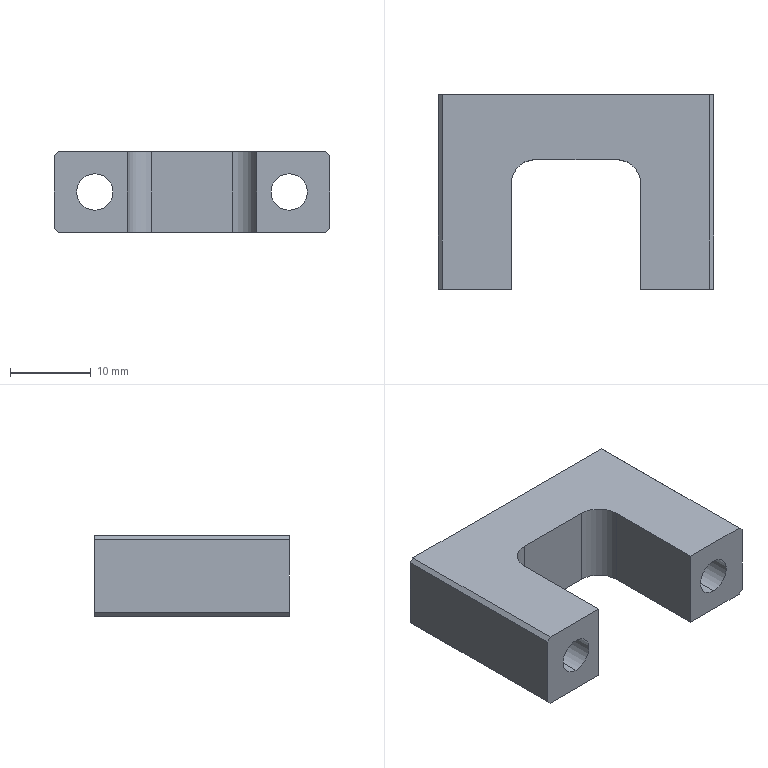Part | SolidWorks | features BaseBody 1 | 1 solid | 26 faces | box 34 x 24 x 10 mm | volume 4547 mm3 | plane 16 | cylinder 10 | commonest cylinder face diameters 4.5 x4 8 x4 6 x2
STEP:
#1=CARTESIAN_POINT('',(-12.,-4.6,-4.));
#2=VERTEX_POINT('',#1);
#3=CARTESIAN_POINT('',(-12.,-4.6,4.));
#4=VERTEX_POINT('',#3);
#5=CARTESIAN_POINT('',(-12.,-4.6,0.));
#6=DIRECTION('',(0.,1.,0.));
#7=DIRECTION('',(0.,0.,1.));
#8=AXIS2_PLACEMENT_3D('',#5,#6,#7);
#9=CIRCLE('',#8,4.);
#10=EDGE_CURVE('',#2,#4,#9,.T.);
#11=ORIENTED_EDGE('',*,*,#10,.F.);
#12=CARTESIAN_POINT('',(-12.,0.,-4.));
#13=VERTEX_POINT('',#12);
#14=CARTESIAN_POINT('',(-12.,0.,-4.));
#15=DIRECTION('',(0.,1.,0.));
#16=VECTOR('',#15,1000.);
#17=LINE('',#14,#16);
#18=EDGE_CURVE('',#2,#13,#17,.T.);
#19=ORIENTED_EDGE('',*,*,#18,.T.);
#20=CARTESIAN_POINT('',(-12.,0.,4.));
#21=VERTEX_POINT('',#20);
#22=CARTESIAN_POINT('',(-12.,0.,0.));
#23=DIRECTION('',(0.,1.,0.));
#24=DIRECTION('',(0.,0.,1.));
#25=AXIS2_PLACEMENT_3D('',#22,#23,#24);
#26=CIRCLE('',#25,4.);
#27=EDGE_CURVE('',#13,#21,#26,.T.);
#28=ORIENTED_EDGE('',*,*,#27,.T.);
#29=CARTESIAN_POINT('',(-12.,0.,4.));
#30=DIRECTION('',(0.,1.,0.));
#31=VECTOR('',#30,1000.);
#32=LINE('',#29,#31);
#33=EDGE_CURVE('',#4,#21,#32,.T.);
#34=ORIENTED_EDGE('',*,*,#33,.F.);
#35=EDGE_LOOP('',(#11,#19,#28,#34));
#36=FACE_OUTER_BOUND('',#35,.T.);
#37=CARTESIAN_POINT('',(-12.,0.,0.));
#38=DIRECTION('',(0.,1.,0.));
#39=DIRECTION('',(0.,0.,1.));
#40=AXIS2_PLACEMENT_3D('',#37,#38,#39);
#41=CYLINDRICAL_SURFACE('',#40,4.);
#42=ADVANCED_FACE('',(#36),#41,.F.);
#43=CARTESIAN_POINT('',(-12.,-24.,-2.25));
#44=VERTEX_POINT('',#43);
#45=CARTESIAN_POINT('',(-12.,-24.,2.25));
#46=VERTEX_POINT('',#45);
#47=CARTESIAN_POINT('',(-12.,-24.,0.));
#48=DIRECTION('',(0.,1.,0.));
#49=DIRECTION('',(-1.,0.,0.));
#50=AXIS2_PLACEMENT_3D('',#47,#48,#49);
#51=CIRCLE('',#50,2.25);
#52=EDGE_CURVE('',#44,#46,#51,.T.);
#53=ORIENTED_EDGE('',*,*,#52,.F.);
#54=CARTESIAN_POINT('',(-12.,-4.6,-2.25));
#55=VERTEX_POINT('',#54);
#56=CARTESIAN_POINT('',(-12.,0.,-2.25));
#57=DIRECTION('',(0.,1.,0.));
#58=VECTOR('',#57,1000.);
#59=LINE('',#56,#58);
#60=EDGE_CURVE('',#44,#55,#59,.T.);
#61=ORIENTED_EDGE('',*,*,#60,.T.);
#62=CARTESIAN_POINT('',(-12.,-4.6,2.25));
#63=VERTEX_POINT('',#62);
#64=CARTESIAN_POINT('',(-12.,-4.6,0.));
#65=DIRECTION('',(0.,1.,0.));
#66=DIRECTION('',(0.,0.,1.));
#67=AXIS2_PLACEMENT_3D('',#64,#65,#66);
#68=CIRCLE('',#67,2.25);
#69=EDGE_CURVE('',#55,#63,#68,.T.);
#70=ORIENTED_EDGE('',*,*,#69,.T.);
#71=CARTESIAN_POINT('',(-12.,0.,2.25));
#72=DIRECTION('',(0.,1.,0.));
#73=VECTOR('',#72,1000.);
#74=LINE('',#71,#73);
#75=EDGE_CURVE('',#46,#63,#74,.T.);
#76=ORIENTED_EDGE('',*,*,#75,.F.);
#77=EDGE_LOOP('',(#53,#61,#70,#76));
#78=FACE_OUTER_BOUND('',#77,.T.);
#79=CARTESIAN_POINT('',(-12.,0.,0.));
#80=DIRECTION('',(0.,1.,0.));
#81=DIRECTION('',(0.,0.,1.));
#82=AXIS2_PLACEMENT_3D('',#79,#80,#81);
#83=CYLINDRICAL_SURFACE('',#82,2.25);
#84=ADVANCED_FACE('',(#78),#83,.F.);
#85=CARTESIAN_POINT('',(12.,-4.6,-4.));
#86=VERTEX_POINT('',#85);
#87=CARTESIAN_POINT('',(12.,-4.6,4.));
#88=VERTEX_POINT('',#87);
#89=CARTESIAN_POINT('',(12.,-4.6,0.));
#90=DIRECTION('',(0.,1.,0.));
#91=DIRECTION('',(0.,0.,1.));
#92=AXIS2_PLACEMENT_3D('',#89,#90,#91);
#93=CIRCLE('',#92,4.);
#94=EDGE_CURVE('',#86,#88,#93,.T.);
#95=ORIENTED_EDGE('',*,*,#94,.F.);
#96=CARTESIAN_POINT('',(12.,0.,-4.));
#97=VERTEX_POINT('',#96);
#98=CARTESIAN_POINT('',(12.,0.,-4.));
#99=DIRECTION('',(0.,1.,0.));
#100=VECTOR('',#99,1000.);
#101=LINE('',#98,#100);
#102=EDGE_CURVE('',#86,#97,#101,.T.);
#103=ORIENTED_EDGE('',*,*,#102,.T.);
#104=CARTESIAN_POINT('',(12.,0.,4.));
#105=VERTEX_POINT('',#104);
#106=CARTESIAN_POINT('',(12.,0.,0.));
#107=DIRECTION('',(0.,1.,0.));
#108=DIRECTION('',(0.,0.,1.));
#109=AXIS2_PLACEMENT_3D('',#106,#107,#108);
#110=CIRCLE('',#109,4.);
#111=EDGE_CURVE('',#97,#105,#110,.T.);
#112=ORIENTED_EDGE('',*,*,#111,.T.);
#113=CARTESIAN_POINT('',(12.,0.,4.));
#114=DIRECTION('',(0.,1.,0.));
#115=VECTOR('',#114,1000.);
#116=LINE('',#113,#115);
#117=EDGE_CURVE('',#88,#105,#116,.T.);
#118=ORIENTED_EDGE('',*,*,#117,.F.);
#119=EDGE_LOOP('',(#95,#103,#112,#118));
#120=FACE_OUTER_BOUND('',#119,.T.);
#121=CARTESIAN_POINT('',(12.,0.,0.));
#122=DIRECTION('',(0.,1.,0.));
#123=DIRECTION('',(0.,0.,1.));
#124=AXIS2_PLACEMENT_3D('',#121,#122,#123);
#125=CYLINDRICAL_SURFACE('',#124,4.);
#126=ADVANCED_FACE('',(#120),#125,.F.);
#127=CARTESIAN_POINT('',(12.,-24.,-2.25));
#128=VERTEX_POINT('',#127);
#129=CARTESIAN_POINT('',(12.,-24.,2.25));
#130=VERTEX_POINT('',#129);
#131=CARTESIAN_POINT('',(12.,-24.,0.));
#132=DIRECTION('',(0.,1.,0.));
#133=DIRECTION('',(-1.,0.,0.));
#134=AXIS2_PLACEMENT_3D('',#131,#132,#133);
#135=CIRCLE('',#134,2.25);
#136=EDGE_CURVE('',#128,#130,#135,.T.);
#137=ORIENTED_EDGE('',*,*,#136,.F.);
#138=CARTESIAN_POINT('',(12.,-4.6,-2.25));
#139=VERTEX_POINT('',#138);
#140=CARTESIAN_POINT('',(12.,0.,-2.25));
#141=DIRECTION('',(0.,1.,0.));
#142=VECTOR('',#141,1000.);
#143=LINE('',#140,#142);
#144=EDGE_CURVE('',#128,#139,#143,.T.);
#145=ORIENTED_EDGE('',*,*,#144,.T.);
#146=CARTESIAN_POINT('',(12.,-4.6,2.25));
#147=VERTEX_POINT('',#146);
#148=CARTESIAN_POINT('',(12.,-4.6,0.));
#149=DIRECTION('',(0.,1.,0.));
#150=DIRECTION('',(0.,0.,1.));
#151=AXIS2_PLACEMENT_3D('',#148,#149,#150);
#152=CIRCLE('',#151,2.25);
#153=EDGE_CURVE('',#139,#147,#152,.T.);
#154=ORIENTED_EDGE('',*,*,#153,.T.);
#155=CARTESIAN_POINT('',(12.,0.,2.25));
#156=DIRECTION('',(0.,1.,0.));
#157=VECTOR('',#156,1000.);
#158=LINE('',#155,#157);
#159=EDGE_CURVE('',#130,#147,#158,.T.);
#160=ORIENTED_EDGE('',*,*,#159,.F.);
#161=EDGE_LOOP('',(#137,#145,#154,#160));
#162=FACE_OUTER_BOUND('',#161,.T.);
#163=CARTESIAN_POINT('',(12.,0.,0.));
#164=DIRECTION('',(0.,1.,0.));
#165=DIRECTION('',(0.,0.,1.));
#166=AXIS2_PLACEMENT_3D('',#163,#164,#165);
#167=CYLINDRICAL_SURFACE('',#166,2.25);
#168=ADVANCED_FACE('',(#162),#167,.F.);
#169=CARTESIAN_POINT('',(-8.,-11.,5.));
#170=VERTEX_POINT('',#169);
#171=CARTESIAN_POINT('',(-5.,-8.,5.));
#172=VERTEX_POINT('',#171);
#173=CARTESIAN_POINT('',(-5.,-11.,5.));
#174=DIRECTION('',(0.,0.,-1.));
#175=DIRECTION('',(-1.,0.,0.));
#176=AXIS2_PLACEMENT_3D('',#173,#174,#175);
#177=CIRCLE('',#176,3.);
#178=EDGE_CURVE('',#170,#172,#177,.T.);
#179=ORIENTED_EDGE('',*,*,#178,.F.);
#180=CARTESIAN_POINT('',(-8.,-11.,-5.));
#181=VERTEX_POINT('',#180);
#182=CARTESIAN_POINT('',(-8.,-11.,5.));
#183=DIRECTION('',(0.,0.,1.));
#184=VECTOR('',#183,1000.);
#185=LINE('',#182,#184);
#186=EDGE_CURVE('',#181,#170,#185,.T.);
#187=ORIENTED_EDGE('',*,*,#186,.F.);
#188=CARTESIAN_POINT('',(-5.,-8.,-5.));
#189=VERTEX_POINT('',#188);
#190=CARTESIAN_POINT('',(-5.,-11.,-5.));
#191=DIRECTION('',(0.,0.,1.));
#192=DIRECTION('',(-1.,0.,0.));
#193=AXIS2_PLACEMENT_3D('',#190,#191,#192);
#194=CIRCLE('',#193,3.);
#195=EDGE_CURVE('',#189,#181,#194,.T.);
#196=ORIENTED_EDGE('',*,*,#195,.F.);
#197=CARTESIAN_POINT('',(-5.,-8.,-5.));
#198=DIRECTION('',(0.,0.,-1.));
#199=VECTOR('',#198,1000.);
#200=LINE('',#197,#199);
#201=EDGE_CURVE('',#172,#189,#200,.T.);
#202=ORIENTED_EDGE('',*,*,#201,.F.);
#203=EDGE_LOOP('',(#179,#187,#196,#202));
#204=FACE_OUTER_BOUND('',#203,.T.);
#205=CARTESIAN_POINT('',(-5.,-11.,5.));
#206=DIRECTION('',(0.,0.,1.));
#207=DIRECTION('',(1.,0.,0.));
#208=AXIS2_PLACEMENT_3D('',#205,#206,#207);
#209=CYLINDRICAL_SURFACE('',#208,3.);
#210=ADVANCED_FACE('',(#204),#209,.F.);
#211=CARTESIAN_POINT('',(5.,-8.,5.));
#212=VERTEX_POINT('',#211);
#213=CARTESIAN_POINT('',(8.,-11.,5.));
#214=VERTEX_POINT('',#213);
#215=CARTESIAN_POINT('',(5.,-11.,5.));
#216=DIRECTION('',(0.,0.,-1.));
#217=DIRECTION('',(-1.,0.,0.));
#218=AXIS2_PLACEMENT_3D('',#215,#216,#217);
#219=CIRCLE('',#218,3.);
#220=EDGE_CURVE('',#212,#214,#219,.T.);
#221=ORIENTED_EDGE('',*,*,#220,.F.);
#222=CARTESIAN_POINT('',(5.,-8.,-5.));
#223=VERTEX_POINT('',#222);
#224=CARTESIAN_POINT('',(5.,-8.,5.));
#225=DIRECTION('',(0.,0.,1.));
#226=VECTOR('',#225,1000.);
#227=LINE('',#224,#226);
#228=EDGE_CURVE('',#223,#212,#227,.T.);
#229=ORIENTED_EDGE('',*,*,#228,.F.);
#230=CARTESIAN_POINT('',(8.,-11.,-5.));
#231=VERTEX_POINT('',#230);
#232=CARTESIAN_POINT('',(5.,-11.,-5.));
#233=DIRECTION('',(0.,0.,1.));
#234=DIRECTION('',(-1.,0.,0.));
#235=AXIS2_PLACEMENT_3D('',#232,#233,#234);
#236=CIRCLE('',#235,3.);
#237=EDGE_CURVE('',#231,#223,#236,.T.);
#238=ORIENTED_EDGE('',*,*,#237,.F.);
#239=CARTESIAN_POINT('',(8.,-11.,-5.));
#240=DIRECTION('',(0.,0.,-1.));
#241=VECTOR('',#240,1000.);
#242=LINE('',#239,#241);
#243=EDGE_CURVE('',#214,#231,#242,.T.);
#244=ORIENTED_EDGE('',*,*,#243,.F.);
#245=EDGE_LOOP('',(#221,#229,#238,#244));
#246=FACE_OUTER_BOUND('',#245,.T.);
#247=CARTESIAN_POINT('',(5.,-11.,5.));
#248=DIRECTION('',(0.,0.,1.));
#249=DIRECTION('',(1.,0.,0.));
#250=AXIS2_PLACEMENT_3D('',#247,#248,#249);
#251=CYLINDRICAL_SURFACE('',#250,3.);
#252=ADVANCED_FACE('',(#246),#251,.F.);
#253=CARTESIAN_POINT('',(-17.,0.,4.5));
#254=VERTEX_POINT('',#253);
#255=CARTESIAN_POINT('',(-16.5,0.,5.));
#256=VERTEX_POINT('',#255);
#257=CARTESIAN_POINT('',(-16.5,0.,5.));
#258=DIRECTION('',(0.7071,0.,0.7071));
#259=VECTOR('',#258,1000.);
#260=LINE('',#257,#259);
#261=EDGE_CURVE('',#254,#256,#260,.T.);
#262=ORIENTED_EDGE('',*,*,#261,.F.);
#263=CARTESIAN_POINT('',(-17.,-24.,4.5));
#264=VERTEX_POINT('',#263);
#265=CARTESIAN_POINT('',(-17.,-24.,4.5));
#266=DIRECTION('',(0.,1.,0.));
#267=VECTOR('',#266,1000.);
#268=LINE('',#265,#267);
#269=EDGE_CURVE('',#264,#254,#268,.T.);
#270=ORIENTED_EDGE('',*,*,#269,.F.);
#271=CARTESIAN_POINT('',(-16.5,-24.,5.));
#272=VERTEX_POINT('',#271);
#273=CARTESIAN_POINT('',(-16.5,-24.,5.));
#274=DIRECTION('',(-0.7071,0.,-0.7071));
#275=VECTOR('',#274,1000.);
#276=LINE('',#273,#275);
#277=EDGE_CURVE('',#272,#264,#276,.T.);
#278=ORIENTED_EDGE('',*,*,#277,.F.);
#279=CARTESIAN_POINT('',(-16.5,0.,5.));
#280=DIRECTION('',(0.,-1.,0.));
#281=VECTOR('',#280,1000.);
#282=LINE('',#279,#281);
#283=EDGE_CURVE('',#256,#272,#282,.T.);
#284=ORIENTED_EDGE('',*,*,#283,.F.);
#285=EDGE_LOOP('',(#262,#270,#278,#284));
#286=FACE_OUTER_BOUND('',#285,.T.);
#287=CARTESIAN_POINT('',(-16.5,0.,5.));
#288=DIRECTION('',(0.7071,0.,-0.7071));
#289=DIRECTION('',(0.,-1.,0.));
#290=AXIS2_PLACEMENT_3D('',#287,#288,#289);
#291=PLANE('',#290);
#292=ADVANCED_FACE('',(#286),#291,.F.);
#293=CARTESIAN_POINT('',(-16.5,0.,-5.));
#294=VERTEX_POINT('',#293);
#295=CARTESIAN_POINT('',(-17.,0.,-4.5));
#296=VERTEX_POINT('',#295);
#297=CARTESIAN_POINT('',(-17.,0.,-4.5));
#298=DIRECTION('',(-0.7071,0.,0.7071));
#299=VECTOR('',#298,1000.);
#300=LINE('',#297,#299);
#301=EDGE_CURVE('',#294,#296,#300,.T.);
#302=ORIENTED_EDGE('',*,*,#301,.F.);
#303=CARTESIAN_POINT('',(-16.5,-24.,-5.));
#304=VERTEX_POINT('',#303);
#305=CARTESIAN_POINT('',(-16.5,0.,-5.));
#306=DIRECTION('',(0.,1.,0.));
#307=VECTOR('',#306,1000.);
#308=LINE('',#305,#307);
#309=EDGE_CURVE('',#304,#294,#308,.T.);
#310=ORIENTED_EDGE('',*,*,#309,.F.);
#311=CARTESIAN_POINT('',(-17.,-24.,-4.5));
#312=VERTEX_POINT('',#311);
#313=CARTESIAN_POINT('',(-17.,-24.,-4.5));
#314=DIRECTION('',(0.7071,0.,-0.7071));
#315=VECTOR('',#314,1000.);
#316=LINE('',#313,#315);
#317=EDGE_CURVE('',#312,#304,#316,.T.);
#318=ORIENTED_EDGE('',*,*,#317,.F.);
#319=CARTESIAN_POINT('',(-17.,-24.,-4.5));
#320=DIRECTION('',(0.,-1.,0.));
#321=VECTOR('',#320,1000.);
#322=LINE('',#319,#321);
#323=EDGE_CURVE('',#296,#312,#322,.T.);
#324=ORIENTED_EDGE('',*,*,#323,.F.);
#325=EDGE_LOOP('',(#302,#310,#318,#324));
#326=FACE_OUTER_BOUND('',#325,.T.);
#327=CARTESIAN_POINT('',(-17.,-24.,-4.5));
#328=DIRECTION('',(-0.7071,0.,-0.7071));
#329=DIRECTION('',(-0.7071,0.,0.7071));
#330=AXIS2_PLACEMENT_3D('',#327,#328,#329);
#331=PLANE('',#330);
#332=ADVANCED_FACE('',(#326),#331,.T.);
#333=CARTESIAN_POINT('',(17.,-24.,4.5));
#334=VERTEX_POINT('',#333);
#335=CARTESIAN_POINT('',(16.5,-24.,5.));
#336=VERTEX_POINT('',#335);
#337=CARTESIAN_POINT('',(16.5,-24.,5.));
#338=DIRECTION('',(-0.7071,0.,0.7071));
#339=VECTOR('',#338,1000.);
#340=LINE('',#337,#339);
#341=EDGE_CURVE('',#334,#336,#340,.T.);
#342=ORIENTED_EDGE('',*,*,#341,.F.);
#343=CARTESIAN_POINT('',(17.,0.,4.5));
#344=VERTEX_POINT('',#343);
#345=CARTESIAN_POINT('',(17.,0.,4.5));
#346=DIRECTION('',(0.,-1.,0.));
#347=VECTOR('',#346,1000.);
#348=LINE('',#345,#347);
#349=EDGE_CURVE('',#344,#334,#348,.T.);
#350=ORIENTED_EDGE('',*,*,#349,.F.);
#351=CARTESIAN_POINT('',(16.5,0.,5.));
#352=VERTEX_POINT('',#351);
#353=CARTESIAN_POINT('',(16.5,0.,5.));
#354=DIRECTION('',(0.7071,0.,-0.7071));
#355=VECTOR('',#354,1000.);
#356=LINE('',#353,#355);
#357=EDGE_CURVE('',#352,#344,#356,.T.);
#358=ORIENTED_EDGE('',*,*,#357,.F.);
#359=CARTESIAN_POINT('',(16.5,0.,5.));
#360=DIRECTION('',(0.,1.,0.));
#361=VECTOR('',#360,1000.);
#362=LINE('',#359,#361);
#363=EDGE_CURVE('',#336,#352,#362,.T.);
#364=ORIENTED_EDGE('',*,*,#363,.F.);
#365=EDGE_LOOP('',(#342,#350,#358,#364));
#366=FACE_OUTER_BOUND('',#365,.T.);
#367=CARTESIAN_POINT('',(16.5,0.,5.));
#368=DIRECTION('',(-0.7071,0.,-0.7071));
#369=DIRECTION('',(-0.7071,0.,0.7071));
#370=AXIS2_PLACEMENT_3D('',#367,#368,#369);
#371=PLANE('',#370);
#372=ADVANCED_FACE('',(#366),#371,.F.);
#373=CARTESIAN_POINT('',(16.5,-24.,-5.));
#374=VERTEX_POINT('',#373);
#375=CARTESIAN_POINT('',(17.,-24.,-4.5));
#376=VERTEX_POINT('',#375);
#377=CARTESIAN_POINT('',(17.,-24.,-4.5));
#378=DIRECTION('',(0.7071,0.,0.7071));
#379=VECTOR('',#378,1000.);
#380=LINE('',#377,#379);
#381=EDGE_CURVE('',#374,#376,#380,.T.);
#382=ORIENTED_EDGE('',*,*,#381,.F.);
#383=CARTESIAN_POINT('',(16.5,0.,-5.));
#384=VERTEX_POINT('',#383);
#385=CARTESIAN_POINT('',(16.5,-24.,-5.));
#386=DIRECTION('',(0.,-1.,0.));
#387=VECTOR('',#386,1000.);
#388=LINE('',#385,#387);
#389=EDGE_CURVE('',#384,#374,#388,.T.);
#390=ORIENTED_EDGE('',*,*,#389,.F.);
#391=CARTESIAN_POINT('',(17.,0.,-4.5));
#392=VERTEX_POINT('',#391);
#393=CARTESIAN_POINT('',(17.,0.,-4.5));
#394=DIRECTION('',(-0.7071,0.,-0.7071));
#395=VECTOR('',#394,1000.);
#396=LINE('',#393,#395);
#397=EDGE_CURVE('',#392,#384,#396,.T.);
#398=ORIENTED_EDGE('',*,*,#397,.F.);
#399=CARTESIAN_POINT('',(17.,0.,-4.5));
#400=DIRECTION('',(0.,1.,0.));
#401=VECTOR('',#400,1000.);
#402=LINE('',#399,#401);
#403=EDGE_CURVE('',#376,#392,#402,.T.);
#404=ORIENTED_EDGE('',*,*,#403,.F.);
#405=EDGE_LOOP('',(#382,#390,#398,#404));
#406=FACE_OUTER_BOUND('',#405,.T.);
#407=CARTESIAN_POINT('',(17.,0.,-4.5));
#408=DIRECTION('',(0.7071,0.,-0.7071));
#409=DIRECTION('',(0.,-1.,0.));
#410=AXIS2_PLACEMENT_3D('',#407,#408,#409);
#411=PLANE('',#410);
#412=ADVANCED_FACE('',(#406),#411,.T.);
#413=CARTESIAN_POINT('',(-12.,-4.6,0.));
#414=DIRECTION('',(0.,1.,0.));
#415=DIRECTION('',(0.,0.,1.));
#416=AXIS2_PLACEMENT_3D('',#413,#414,#415);
#417=CIRCLE('',#416,2.25);
#418=EDGE_CURVE('',#63,#55,#417,.T.);
#419=ORIENTED_EDGE('',*,*,#418,.F.);
#420=ORIENTED_EDGE('',*,*,#69,.F.);
#421=EDGE_LOOP('',(#419,#420));
#422=FACE_BOUND('',#421,.T.);
#423=CARTESIAN_POINT('',(-12.,-4.6,0.));
#424=DIRECTION('',(0.,1.,0.));
#425=DIRECTION('',(0.,0.,1.));
#426=AXIS2_PLACEMENT_3D('',#423,#424,#425);
#427=CIRCLE('',#426,4.);
#428=EDGE_CURVE('',#4,#2,#427,.T.);
#429=ORIENTED_EDGE('',*,*,#428,.T.);
#430=ORIENTED_EDGE('',*,*,#10,.T.);
#431=EDGE_LOOP('',(#429,#430));
#432=FACE_OUTER_BOUND('',#431,.T.);
#433=CARTESIAN_POINT('',(-9.75,-4.6,0.));
#434=DIRECTION('',(0.,-1.,0.));
#435=DIRECTION('',(0.,0.,-1.));
#436=AXIS2_PLACEMENT_3D('',#433,#434,#435);
#437=PLANE('',#436);
#438=ADVANCED_FACE('',(#422,#432),#437,.F.);
#439=CARTESIAN_POINT('',(12.,-4.6,0.));
#440=DIRECTION('',(0.,1.,0.));
#441=DIRECTION('',(0.,0.,1.));
#442=AXIS2_PLACEMENT_3D('',#439,#440,#441);
#443=CIRCLE('',#442,2.25);
#444=EDGE_CURVE('',#147,#139,#443,.T.);
#445=ORIENTED_EDGE('',*,*,#444,.F.);
#446=ORIENTED_EDGE('',*,*,#153,.F.);
#447=EDGE_LOOP('',(#445,#446));
#448=FACE_BOUND('',#447,.T.);
#449=CARTESIAN_POINT('',(12.,-4.6,0.));
#450=DIRECTION('',(0.,1.,0.));
#451=DIRECTION('',(0.,0.,1.));
#452=AXIS2_PLACEMENT_3D('',#449,#450,#451);
#453=CIRCLE('',#452,4.);
#454=EDGE_CURVE('',#88,#86,#453,.T.);
#455=ORIENTED_EDGE('',*,*,#454,.T.);
#456=ORIENTED_EDGE('',*,*,#94,.T.);
#457=EDGE_LOOP('',(#455,#456));
#458=FACE_OUTER_BOUND('',#457,.T.);
#459=CARTESIAN_POINT('',(14.25,-4.6,0.));
#460=DIRECTION('',(0.,-1.,0.));
#461=DIRECTION('',(0.,0.,-1.));
#462=AXIS2_PLACEMENT_3D('',#459,#460,#461);
#463=PLANE('',#462);
#464=ADVANCED_FACE('',(#448,#458),#463,.F.);
#465=CARTESIAN_POINT('',(-17.,0.,-5.));
#466=DIRECTION('',(-1.,0.,0.));
#467=VECTOR('',#466,1000.);
#468=LINE('',#465,#467);
#469=EDGE_CURVE('',#384,#294,#468,.T.);
#470=ORIENTED_EDGE('',*,*,#469,.F.);
#471=ORIENTED_EDGE('',*,*,#389,.T.);
#472=CARTESIAN_POINT('',(8.,-24.,-5.));
#473=VERTEX_POINT('',#472);
#474=CARTESIAN_POINT('',(17.,-24.,-5.));
#475=DIRECTION('',(1.,0.,0.));
#476=VECTOR('',#475,1000.);
#477=LINE('',#474,#476);
#478=EDGE_CURVE('',#473,#374,#477,.T.);
#479=ORIENTED_EDGE('',*,*,#478,.F.);
#480=CARTESIAN_POINT('',(8.,-24.,-5.));
#481=DIRECTION('',(0.,-1.,0.));
#482=VECTOR('',#481,1000.);
#483=LINE('',#480,#482);
#484=EDGE_CURVE('',#231,#473,#483,.T.);
#485=ORIENTED_EDGE('',*,*,#484,.F.);
#486=ORIENTED_EDGE('',*,*,#237,.T.);
#487=CARTESIAN_POINT('',(8.,-8.,-5.));
#488=DIRECTION('',(1.,0.,0.));
#489=VECTOR('',#488,1000.);
#490=LINE('',#487,#489);
#491=EDGE_CURVE('',#189,#223,#490,.T.);
#492=ORIENTED_EDGE('',*,*,#491,.F.);
#493=ORIENTED_EDGE('',*,*,#195,.T.);
#494=CARTESIAN_POINT('',(-8.,-24.,-5.));
#495=VERTEX_POINT('',#494);
#496=CARTESIAN_POINT('',(-8.,-8.,-5.));
#497=DIRECTION('',(0.,1.,0.));
#498=VECTOR('',#497,1000.);
#499=LINE('',#496,#498);
#500=EDGE_CURVE('',#495,#181,#499,.T.);
#501=ORIENTED_EDGE('',*,*,#500,.F.);
#502=CARTESIAN_POINT('',(-8.,-24.,-5.));
#503=DIRECTION('',(1.,0.,0.));
#504=VECTOR('',#503,1000.);
#505=LINE('',#502,#504);
#506=EDGE_CURVE('',#304,#495,#505,.T.);
#507=ORIENTED_EDGE('',*,*,#506,.F.);
#508=ORIENTED_EDGE('',*,*,#309,.T.);
#509=EDGE_LOOP('',(#470,#471,#479,#485,#486,#492,#493,#501,#507,#508));
#510=FACE_OUTER_BOUND('',#509,.T.);
#511=CARTESIAN_POINT('',(0.,0.,-5.));
#512=DIRECTION('',(0.,0.,-1.));
#513=DIRECTION('',(0.,-1.,0.));
#514=AXIS2_PLACEMENT_3D('',#511,#512,#513);
#515=PLANE('',#514);
#516=ADVANCED_FACE('',(#510),#515,.T.);
#517=CARTESIAN_POINT('',(8.,-24.,5.));
#518=VERTEX_POINT('',#517);
#519=CARTESIAN_POINT('',(17.,-24.,5.));
#520=DIRECTION('',(1.,0.,0.));
#521=VECTOR('',#520,1000.);
#522=LINE('',#519,#521);
#523=EDGE_CURVE('',#518,#336,#522,.T.);
#524=ORIENTED_EDGE('',*,*,#523,.T.);
#525=ORIENTED_EDGE('',*,*,#363,.T.);
#526=CARTESIAN_POINT('',(-17.,0.,5.));
#527=DIRECTION('',(-1.,0.,0.));
#528=VECTOR('',#527,1000.);
#529=LINE('',#526,#528);
#530=EDGE_CURVE('',#352,#256,#529,.T.);
#531=ORIENTED_EDGE('',*,*,#530,.T.);
#532=ORIENTED_EDGE('',*,*,#283,.T.);
#533=CARTESIAN_POINT('',(-8.,-24.,5.));
#534=VERTEX_POINT('',#533);
#535=CARTESIAN_POINT('',(-8.,-24.,5.));
#536=DIRECTION('',(1.,0.,0.));
#537=VECTOR('',#536,1000.);
#538=LINE('',#535,#537);
#539=EDGE_CURVE('',#272,#534,#538,.T.);
#540=ORIENTED_EDGE('',*,*,#539,.T.);
#541=CARTESIAN_POINT('',(-8.,-8.,5.));
#542=DIRECTION('',(0.,1.,0.));
#543=VECTOR('',#542,1000.);
#544=LINE('',#541,#543);
#545=EDGE_CURVE('',#534,#170,#544,.T.);
#546=ORIENTED_EDGE('',*,*,#545,.T.);
#547=ORIENTED_EDGE('',*,*,#178,.T.);
#548=CARTESIAN_POINT('',(8.,-8.,5.));
#549=DIRECTION('',(1.,0.,0.));
#550=VECTOR('',#549,1000.);
#551=LINE('',#548,#550);
#552=EDGE_CURVE('',#172,#212,#551,.T.);
#553=ORIENTED_EDGE('',*,*,#552,.T.);
#554=ORIENTED_EDGE('',*,*,#220,.T.);
#555=CARTESIAN_POINT('',(8.,-24.,5.));
#556=DIRECTION('',(0.,-1.,0.));
#557=VECTOR('',#556,1000.);
#558=LINE('',#555,#557);
#559=EDGE_CURVE('',#214,#518,#558,.T.);
#560=ORIENTED_EDGE('',*,*,#559,.T.);
#561=EDGE_LOOP('',(#524,#525,#531,#532,#540,#546,#547,#553,#554,#560));
#562=FACE_OUTER_BOUND('',#561,.T.);
#563=CARTESIAN_POINT('',(0.,0.,5.));
#564=DIRECTION('',(0.,0.,-1.));
#565=DIRECTION('',(0.,-1.,0.));
#566=AXIS2_PLACEMENT_3D('',#563,#564,#565);
#567=PLANE('',#566);
#568=ADVANCED_FACE('',(#562),#567,.F.);
#569=CARTESIAN_POINT('',(-17.,0.,5.));
#570=DIRECTION('',(0.,0.,-1.));
#571=VECTOR('',#570,1000.);
#572=LINE('',#569,#571);
#573=EDGE_CURVE('',#254,#296,#572,.T.);
#574=ORIENTED_EDGE('',*,*,#573,.T.);
#575=ORIENTED_EDGE('',*,*,#323,.T.);
#576=CARTESIAN_POINT('',(-17.,-24.,5.));
#577=DIRECTION('',(0.,0.,-1.));
#578=VECTOR('',#577,1000.);
#579=LINE('',#576,#578);
#580=EDGE_CURVE('',#264,#312,#579,.T.);
#581=ORIENTED_EDGE('',*,*,#580,.F.);
#582=ORIENTED_EDGE('',*,*,#269,.T.);
#583=EDGE_LOOP('',(#574,#575,#581,#582));
#584=FACE_OUTER_BOUND('',#583,.T.);
#585=CARTESIAN_POINT('',(-17.,-24.,5.));
#586=DIRECTION('',(1.,0.,0.));
#587=DIRECTION('',(0.,1.,0.));
#588=AXIS2_PLACEMENT_3D('',#585,#586,#587);
#589=PLANE('',#588);
#590=ADVANCED_FACE('',(#584),#589,.F.);
#591=CARTESIAN_POINT('',(12.,0.,0.));
#592=DIRECTION('',(0.,1.,0.));
#593=DIRECTION('',(0.,0.,1.));
#594=AXIS2_PLACEMENT_3D('',#591,#592,#593);
#595=CIRCLE('',#594,4.);
#596=EDGE_CURVE('',#105,#97,#595,.T.);
#597=ORIENTED_EDGE('',*,*,#596,.F.);
#598=ORIENTED_EDGE('',*,*,#111,.F.);
#599=EDGE_LOOP('',(#597,#598));
#600=FACE_BOUND('',#599,.T.);
#601=CARTESIAN_POINT('',(-12.,0.,0.));
#602=DIRECTION('',(0.,1.,0.));
#603=DIRECTION('',(0.,0.,1.));
#604=AXIS2_PLACEMENT_3D('',#601,#602,#603);
#605=CIRCLE('',#604,4.);
#606=EDGE_CURVE('',#21,#13,#605,.T.);
#607=ORIENTED_EDGE('',*,*,#606,.F.);
#608=ORIENTED_EDGE('',*,*,#27,.F.);
#609=EDGE_LOOP('',(#607,#608));
#610=FACE_BOUND('',#609,.T.);
#611=CARTESIAN_POINT('',(17.,0.,5.));
#612=DIRECTION('',(0.,0.,-1.));
#613=VECTOR('',#612,1000.);
#614=LINE('',#611,#613);
#615=EDGE_CURVE('',#344,#392,#614,.T.);
#616=ORIENTED_EDGE('',*,*,#615,.T.);
#617=ORIENTED_EDGE('',*,*,#397,.T.);
#618=ORIENTED_EDGE('',*,*,#469,.T.);
#619=ORIENTED_EDGE('',*,*,#301,.T.);
#620=ORIENTED_EDGE('',*,*,#573,.F.);
#621=ORIENTED_EDGE('',*,*,#261,.T.);
#622=ORIENTED_EDGE('',*,*,#530,.F.);
#623=ORIENTED_EDGE('',*,*,#357,.T.);
#624=EDGE_LOOP('',(#616,#617,#618,#619,#620,#621,#622,#623));
#625=FACE_OUTER_BOUND('',#624,.T.);
#626=CARTESIAN_POINT('',(-17.,0.,5.));
#627=DIRECTION('',(0.,-1.,0.));
#628=DIRECTION('',(0.,0.,-1.));
#629=AXIS2_PLACEMENT_3D('',#626,#627,#628);
#630=PLANE('',#629);
#631=ADVANCED_FACE('',(#600,#610,#625),#630,.F.);
#632=CARTESIAN_POINT('',(17.,-24.,5.));
#633=DIRECTION('',(0.,0.,-1.));
#634=VECTOR('',#633,1000.);
#635=LINE('',#632,#634);
#636=EDGE_CURVE('',#334,#376,#635,.T.);
#637=ORIENTED_EDGE('',*,*,#636,.T.);
#638=ORIENTED_EDGE('',*,*,#403,.T.);
#639=ORIENTED_EDGE('',*,*,#615,.F.);
#640=ORIENTED_EDGE('',*,*,#349,.T.);
#641=EDGE_LOOP('',(#637,#638,#639,#640));
#642=FACE_OUTER_BOUND('',#641,.T.);
#643=CARTESIAN_POINT('',(17.,0.,5.));
#644=DIRECTION('',(-1.,0.,0.));
#645=DIRECTION('',(0.,0.,1.));
#646=AXIS2_PLACEMENT_3D('',#643,#644,#645);
#647=PLANE('',#646);
#648=ADVANCED_FACE('',(#642),#647,.F.);
#649=CARTESIAN_POINT('',(12.,-24.,0.));
#650=DIRECTION('',(0.,1.,0.));
#651=DIRECTION('',(-1.,0.,0.));
#652=AXIS2_PLACEMENT_3D('',#649,#650,#651);
#653=CIRCLE('',#652,2.25);
#654=EDGE_CURVE('',#130,#128,#653,.T.);
#655=ORIENTED_EDGE('',*,*,#654,.T.);
#656=ORIENTED_EDGE('',*,*,#136,.T.);
#657=EDGE_LOOP('',(#655,#656));
#658=FACE_BOUND('',#657,.T.);
#659=ORIENTED_EDGE('',*,*,#478,.T.);
#660=ORIENTED_EDGE('',*,*,#381,.T.);
#661=ORIENTED_EDGE('',*,*,#636,.F.);
#662=ORIENTED_EDGE('',*,*,#341,.T.);
#663=ORIENTED_EDGE('',*,*,#523,.F.);
#664=CARTESIAN_POINT('',(8.,-24.,5.));
#665=DIRECTION('',(0.,0.,-1.));
#666=VECTOR('',#665,1000.);
#667=LINE('',#664,#666);
#668=EDGE_CURVE('',#518,#473,#667,.T.);
#669=ORIENTED_EDGE('',*,*,#668,.T.);
#670=EDGE_LOOP('',(#659,#660,#661,#662,#663,#669));
#671=FACE_OUTER_BOUND('',#670,.T.);
#672=CARTESIAN_POINT('',(17.,-24.,5.));
#673=DIRECTION('',(0.,1.,0.));
#674=DIRECTION('',(1.,0.,0.));
#675=AXIS2_PLACEMENT_3D('',#672,#673,#674);
#676=PLANE('',#675);
#677=ADVANCED_FACE('',(#658,#671),#676,.F.);
#678=ORIENTED_EDGE('',*,*,#559,.F.);
#679=ORIENTED_EDGE('',*,*,#243,.T.);
#680=ORIENTED_EDGE('',*,*,#484,.T.);
#681=ORIENTED_EDGE('',*,*,#668,.F.);
#682=EDGE_LOOP('',(#678,#679,#680,#681));
#683=FACE_OUTER_BOUND('',#682,.T.);
#684=CARTESIAN_POINT('',(8.,-24.,5.));
#685=DIRECTION('',(1.,0.,0.));
#686=DIRECTION('',(0.,1.,0.));
#687=AXIS2_PLACEMENT_3D('',#684,#685,#686);
#688=PLANE('',#687);
#689=ADVANCED_FACE('',(#683),#688,.F.);
#690=ORIENTED_EDGE('',*,*,#491,.T.);
#691=ORIENTED_EDGE('',*,*,#228,.T.);
#692=ORIENTED_EDGE('',*,*,#552,.F.);
#693=ORIENTED_EDGE('',*,*,#201,.T.);
#694=EDGE_LOOP('',(#690,#691,#692,#693));
#695=FACE_OUTER_BOUND('',#694,.T.);
#696=CARTESIAN_POINT('',(8.,-8.,5.));
#697=DIRECTION('',(0.,1.,0.));
#698=DIRECTION('',(1.,0.,0.));
#699=AXIS2_PLACEMENT_3D('',#696,#697,#698);
#700=PLANE('',#699);
#701=ADVANCED_FACE('',(#695),#700,.F.);
#702=ORIENTED_EDGE('',*,*,#500,.T.);
#703=ORIENTED_EDGE('',*,*,#186,.T.);
#704=ORIENTED_EDGE('',*,*,#545,.F.);
#705=CARTESIAN_POINT('',(-8.,-24.,5.));
#706=DIRECTION('',(0.,0.,-1.));
#707=VECTOR('',#706,1000.);
#708=LINE('',#705,#707);
#709=EDGE_CURVE('',#534,#495,#708,.T.);
#710=ORIENTED_EDGE('',*,*,#709,.T.);
#711=EDGE_LOOP('',(#702,#703,#704,#710));
#712=FACE_OUTER_BOUND('',#711,.T.);
#713=CARTESIAN_POINT('',(-8.,-8.,5.));
#714=DIRECTION('',(-1.,0.,0.));
#715=DIRECTION('',(0.,0.,1.));
#716=AXIS2_PLACEMENT_3D('',#713,#714,#715);
#717=PLANE('',#716);
#718=ADVANCED_FACE('',(#712),#717,.F.);
#719=CARTESIAN_POINT('',(-12.,-24.,0.));
#720=DIRECTION('',(0.,1.,0.));
#721=DIRECTION('',(-1.,0.,0.));
#722=AXIS2_PLACEMENT_3D('',#719,#720,#721);
#723=CIRCLE('',#722,2.25);
#724=EDGE_CURVE('',#46,#44,#723,.T.);
#725=ORIENTED_EDGE('',*,*,#724,.T.);
#726=ORIENTED_EDGE('',*,*,#52,.T.);
#727=EDGE_LOOP('',(#725,#726));
#728=FACE_BOUND('',#727,.T.);
#729=ORIENTED_EDGE('',*,*,#580,.T.);
#730=ORIENTED_EDGE('',*,*,#317,.T.);
#731=ORIENTED_EDGE('',*,*,#506,.T.);
#732=ORIENTED_EDGE('',*,*,#709,.F.);
#733=ORIENTED_EDGE('',*,*,#539,.F.);
#734=ORIENTED_EDGE('',*,*,#277,.T.);
#735=EDGE_LOOP('',(#729,#730,#731,#732,#733,#734));
#736=FACE_OUTER_BOUND('',#735,.T.);
#737=CARTESIAN_POINT('',(-8.,-24.,5.));
#738=DIRECTION('',(0.,1.,0.));
#739=DIRECTION('',(1.,0.,0.));
#740=AXIS2_PLACEMENT_3D('',#737,#738,#739);
#741=PLANE('',#740);
#742=ADVANCED_FACE('',(#728,#736),#741,.F.);
#743=ORIENTED_EDGE('',*,*,#144,.F.);
#744=ORIENTED_EDGE('',*,*,#654,.F.);
#745=ORIENTED_EDGE('',*,*,#159,.T.);
#746=ORIENTED_EDGE('',*,*,#444,.T.);
#747=EDGE_LOOP('',(#743,#744,#745,#746));
#748=FACE_OUTER_BOUND('',#747,.T.);
#749=CARTESIAN_POINT('',(12.,0.,0.));
#750=DIRECTION('',(0.,1.,0.));
#751=DIRECTION('',(0.,0.,1.));
#752=AXIS2_PLACEMENT_3D('',#749,#750,#751);
#753=CYLINDRICAL_SURFACE('',#752,2.25);
#754=ADVANCED_FACE('',(#748),#753,.F.);
#755=ORIENTED_EDGE('',*,*,#102,.F.);
#756=ORIENTED_EDGE('',*,*,#454,.F.);
#757=ORIENTED_EDGE('',*,*,#117,.T.);
#758=ORIENTED_EDGE('',*,*,#596,.T.);
#759=EDGE_LOOP('',(#755,#756,#757,#758));
#760=FACE_OUTER_BOUND('',#759,.T.);
#761=CARTESIAN_POINT('',(12.,0.,0.));
#762=DIRECTION('',(0.,1.,0.));
#763=DIRECTION('',(0.,0.,1.));
#764=AXIS2_PLACEMENT_3D('',#761,#762,#763);
#765=CYLINDRICAL_SURFACE('',#764,4.);
#766=ADVANCED_FACE('',(#760),#765,.F.);
#767=ORIENTED_EDGE('',*,*,#60,.F.);
#768=ORIENTED_EDGE('',*,*,#724,.F.);
#769=ORIENTED_EDGE('',*,*,#75,.T.);
#770=ORIENTED_EDGE('',*,*,#418,.T.);
#771=EDGE_LOOP('',(#767,#768,#769,#770));
#772=FACE_OUTER_BOUND('',#771,.T.);
#773=CARTESIAN_POINT('',(-12.,0.,0.));
#774=DIRECTION('',(0.,1.,0.));
#775=DIRECTION('',(0.,0.,1.));
#776=AXIS2_PLACEMENT_3D('',#773,#774,#775);
#777=CYLINDRICAL_SURFACE('',#776,2.25);
#778=ADVANCED_FACE('',(#772),#777,.F.);
#779=ORIENTED_EDGE('',*,*,#18,.F.);
#780=ORIENTED_EDGE('',*,*,#428,.F.);
#781=ORIENTED_EDGE('',*,*,#33,.T.);
#782=ORIENTED_EDGE('',*,*,#606,.T.);
#783=EDGE_LOOP('',(#779,#780,#781,#782));
#784=FACE_OUTER_BOUND('',#783,.T.);
#785=CARTESIAN_POINT('',(-12.,0.,0.));
#786=DIRECTION('',(0.,1.,0.));
#787=DIRECTION('',(0.,0.,1.));
#788=AXIS2_PLACEMENT_3D('',#785,#786,#787);
#789=CYLINDRICAL_SURFACE('',#788,4.);
#790=ADVANCED_FACE('',(#784),#789,.F.);
#791=CLOSED_SHELL('',(#42,#84,#126,#168,#210,#252,#292,#332,#372,#412,#438,#464,#516,#568,#590,#631,#648,#677,#689,#701,#718,#742,#754,#766,#778,#790));
#792=MANIFOLD_SOLID_BREP('',#791);
#793=CARTESIAN_POINT('',(0.,0.,0.));
#794=DIRECTION('',(0.,0.,1.));
#795=DIRECTION('',(1.,0.,0.));
#796=AXIS2_PLACEMENT_3D('',#793,#794,#795);
#797=(LENGTH_UNIT()NAMED_UNIT(*)SI_UNIT(.MILLI.,.METRE.));
#798=UNCERTAINTY_MEASURE_WITH_UNIT(LENGTH_MEASURE(0.00001),#797,'','');
#799=(NAMED_UNIT(*)PLANE_ANGLE_UNIT()SI_UNIT($,.RADIAN.));
#800=(NAMED_UNIT(*)SI_UNIT($,.STERADIAN.)SOLID_ANGLE_UNIT());
#801=(GEOMETRIC_REPRESENTATION_CONTEXT(3)GLOBAL_UNCERTAINTY_ASSIGNED_CONTEXT((#798))GLOBAL_UNIT_ASSIGNED_CONTEXT((#797,#799,#800))REPRESENTATION_CONTEXT('',''));
#802=ADVANCED_BREP_SHAPE_REPRESENTATION('',(#792,#796),#801);